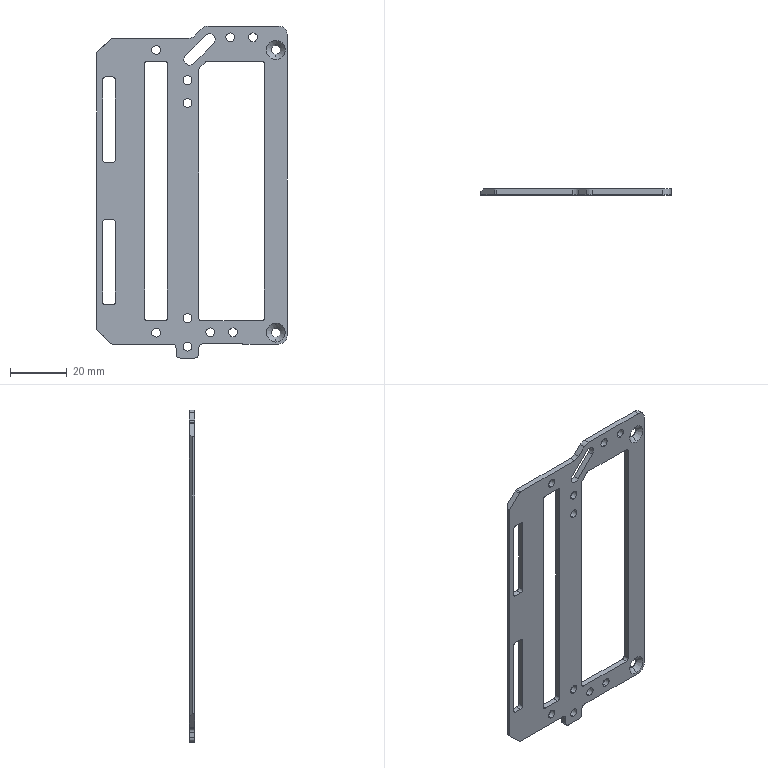Part | SolidWorks | features Fillet 3, Chamfer 2, ICE 2, Extrusion 1, HoleWzd 1 | 1 solid | 94 faces | box 66.8 x 2 x 116.5 mm | volume 8063 mm3 | cylinder 54 | plane 36 | cone 4 | commonest cylinder face diameters 3.1 x20 2 x19 3 x4 3.2 x4 6 x4 4 x3